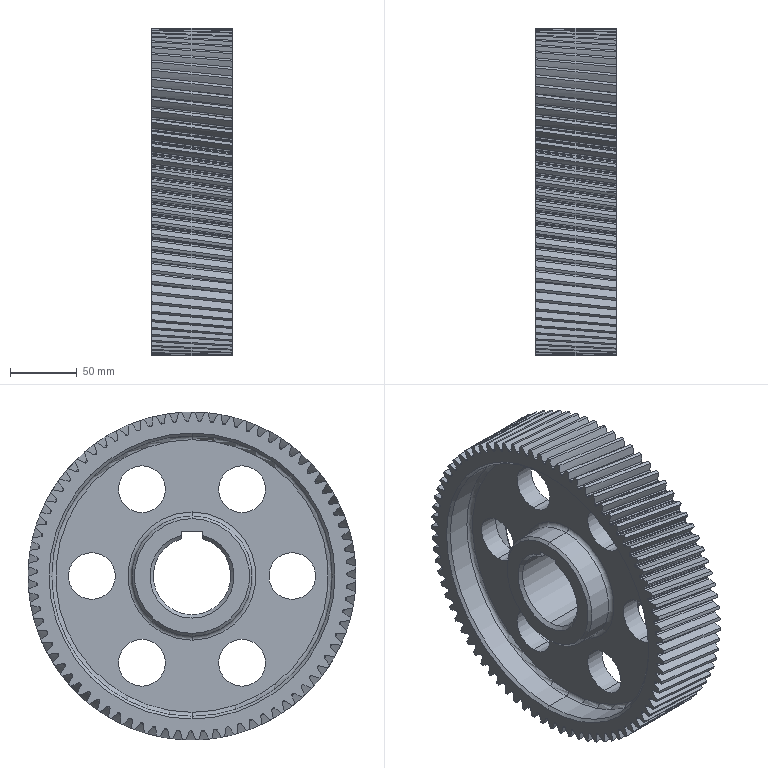Part | SolidWorks | features ICE 6, Chamfer 2, CirPattern 2, Fillet 2, 3DProfileFeature 1, Extrusion 1, Helix 1, HoleWzd 1, MirrorPattern 1, SweepCut 1 | 1 solid | 2030 faces | box 60 x 245.394 x 245.394 mm | volume 1169207 mm3 | plane 1060 | spline 848 | cylinder 103 | cone 11 | torus 8 | commonest cylinder face diameters 245.394 x81 35 x12 90 x4 210 x4 58 x2